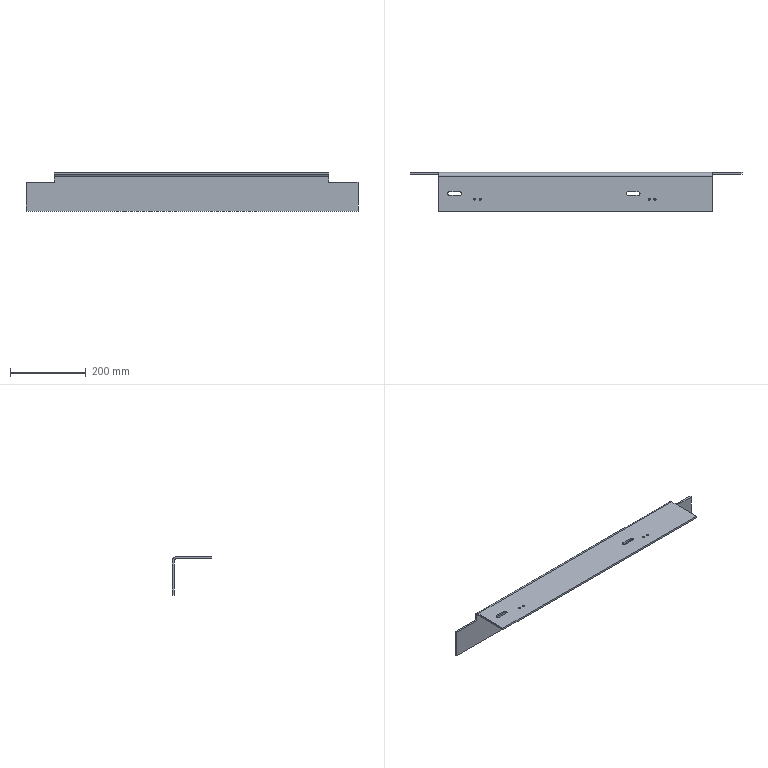Part | NX | 1 solid | 40 faces | box 874.4 x 103.1 x 101 mm | volume 761478 mm3 | plane 16 | cylinder 16 | cone 8 | commonest cylinder face diameters 5 x8 10 x7 20 x1
STEP:
#1=CARTESIAN_POINT('',(669.7,130.8,34.5));
#2=VERTEX_POINT('',#1);
#3=CARTESIAN_POINT('',(669.7,223.9,34.5));
#4=VERTEX_POINT('',#3);
#5=CARTESIAN_POINT('',(669.7,141.246,34.5));
#6=DIRECTION('',(0.,1.,0.));
#7=VECTOR('',#6,1000.);
#8=LINE('',#5,#7);
#9=EDGE_CURVE('',#2,#4,#8,.T.);
#10=ORIENTED_EDGE('',*,*,#9,.F.);
#11=CARTESIAN_POINT('',(669.7,130.8,29.5));
#12=VERTEX_POINT('',#11);
#13=CARTESIAN_POINT('',(669.7,130.8,29.5));
#14=DIRECTION('',(0.,0.,1.));
#15=VECTOR('',#14,1000.);
#16=LINE('',#13,#15);
#17=EDGE_CURVE('',#12,#2,#16,.T.);
#18=ORIENTED_EDGE('',*,*,#17,.F.);
#19=CARTESIAN_POINT('',(669.7,223.9,29.5));
#20=VERTEX_POINT('',#19);
#21=CARTESIAN_POINT('',(669.7,141.246,29.5));
#22=DIRECTION('',(0.,1.,0.));
#23=VECTOR('',#22,1000.);
#24=LINE('',#21,#23);
#25=EDGE_CURVE('',#12,#20,#24,.T.);
#26=ORIENTED_EDGE('',*,*,#25,.T.);
#27=CARTESIAN_POINT('',(669.7,228.9,24.5));
#28=VERTEX_POINT('',#27);
#29=CARTESIAN_POINT('',(669.7,223.9,24.5));
#30=DIRECTION('',(1.,0.,0.));
#31=DIRECTION('',(0.,-1.,0.));
#32=AXIS2_PLACEMENT_3D('',#29,#30,#31);
#33=CIRCLE('',#32,5.);
#34=EDGE_CURVE('',#28,#20,#33,.T.);
#35=ORIENTED_EDGE('',*,*,#34,.F.);
#36=CARTESIAN_POINT('',(669.7,228.9,9.5));
#37=VERTEX_POINT('',#36);
#38=CARTESIAN_POINT('',(669.7,228.9,29.5));
#39=DIRECTION('',(0.,0.,-1.));
#40=VECTOR('',#39,1000.);
#41=LINE('',#38,#40);
#42=EDGE_CURVE('',#28,#37,#41,.T.);
#43=ORIENTED_EDGE('',*,*,#42,.T.);
#44=CARTESIAN_POINT('',(669.7,233.9,9.5));
#45=VERTEX_POINT('',#44);
#46=CARTESIAN_POINT('',(669.7,141.246,9.5));
#47=DIRECTION('',(0.,1.,0.));
#48=VECTOR('',#47,1000.);
#49=LINE('',#46,#48);
#50=EDGE_CURVE('',#37,#45,#49,.T.);
#51=ORIENTED_EDGE('',*,*,#50,.T.);
#52=CARTESIAN_POINT('',(669.7,233.9,24.5));
#53=VERTEX_POINT('',#52);
#54=CARTESIAN_POINT('',(669.7,233.9,29.5));
#55=DIRECTION('',(0.,0.,-1.));
#56=VECTOR('',#55,1000.);
#57=LINE('',#54,#56);
#58=EDGE_CURVE('',#53,#45,#57,.T.);
#59=ORIENTED_EDGE('',*,*,#58,.F.);
#60=CARTESIAN_POINT('',(669.7,223.9,24.5));
#61=DIRECTION('',(1.,0.,0.));
#62=DIRECTION('',(0.,-1.,0.));
#63=AXIS2_PLACEMENT_3D('',#60,#61,#62);
#64=CIRCLE('',#63,10.);
#65=EDGE_CURVE('',#53,#4,#64,.T.);
#66=ORIENTED_EDGE('',*,*,#65,.T.);
#67=EDGE_LOOP('',(#10,#18,#26,#35,#43,#51,#59,#66));
#68=FACE_BOUND('',#67,.T.);
#69=CARTESIAN_POINT('',(669.7,165.9,29.5));
#70=DIRECTION('',(1.,0.,0.));
#71=DIRECTION('',(0.,1.,0.));
#72=AXIS2_PLACEMENT_3D('',#69,#70,#71);
#73=PLANE('',#72);
#74=ADVANCED_FACE('',(#68),#73,.T.);
#75=CARTESIAN_POINT('',(-52.7,130.8,29.5));
#76=VERTEX_POINT('',#75);
#77=CARTESIAN_POINT('',(357.184,130.8,29.5));
#78=DIRECTION('',(1.,0.,0.));
#79=VECTOR('',#78,1000.);
#80=LINE('',#77,#79);
#81=EDGE_CURVE('',#76,#12,#80,.T.);
#82=ORIENTED_EDGE('',*,*,#81,.T.);
#83=ORIENTED_EDGE('',*,*,#17,.T.);
#84=CARTESIAN_POINT('',(-52.7,130.8,34.5));
#85=VERTEX_POINT('',#84);
#86=CARTESIAN_POINT('',(357.184,130.8,34.5));
#87=DIRECTION('',(1.,0.,0.));
#88=VECTOR('',#87,1000.);
#89=LINE('',#86,#88);
#90=EDGE_CURVE('',#85,#2,#89,.T.);
#91=ORIENTED_EDGE('',*,*,#90,.F.);
#92=CARTESIAN_POINT('',(-52.7,130.8,29.5));
#93=DIRECTION('',(0.,0.,-1.));
#94=VECTOR('',#93,1000.);
#95=LINE('',#92,#94);
#96=EDGE_CURVE('',#85,#76,#95,.T.);
#97=ORIENTED_EDGE('',*,*,#96,.T.);
#98=EDGE_LOOP('',(#82,#83,#91,#97));
#99=FACE_BOUND('',#98,.T.);
#100=CARTESIAN_POINT('',(364.7,130.8,29.5));
#101=DIRECTION('',(0.,-1.,0.));
#102=DIRECTION('',(0.,0.,-1.));
#103=AXIS2_PLACEMENT_3D('',#100,#101,#102);
#104=PLANE('',#103);
#105=ADVANCED_FACE('',(#99),#104,.T.);
#106=CARTESIAN_POINT('',(746.7,233.9,9.5));
#107=VERTEX_POINT('',#106);
#108=CARTESIAN_POINT('',(746.7,233.9,-66.5));
#109=VERTEX_POINT('',#108);
#110=CARTESIAN_POINT('',(746.7,233.9,29.5));
#111=DIRECTION('',(0.,0.,-1.));
#112=VECTOR('',#111,1000.);
#113=LINE('',#110,#112);
#114=EDGE_CURVE('',#107,#109,#113,.T.);
#115=ORIENTED_EDGE('',*,*,#114,.F.);
#116=CARTESIAN_POINT('',(746.7,228.9,9.5));
#117=VERTEX_POINT('',#116);
#118=CARTESIAN_POINT('',(746.7,141.246,9.5));
#119=DIRECTION('',(0.,-1.,0.));
#120=VECTOR('',#119,1000.);
#121=LINE('',#118,#120);
#122=EDGE_CURVE('',#107,#117,#121,.T.);
#123=ORIENTED_EDGE('',*,*,#122,.T.);
#124=CARTESIAN_POINT('',(746.7,228.9,-66.5));
#125=VERTEX_POINT('',#124);
#126=CARTESIAN_POINT('',(746.7,228.9,29.5));
#127=DIRECTION('',(0.,0.,-1.));
#128=VECTOR('',#127,1000.);
#129=LINE('',#126,#128);
#130=EDGE_CURVE('',#117,#125,#129,.T.);
#131=ORIENTED_EDGE('',*,*,#130,.T.);
#132=CARTESIAN_POINT('',(746.7,141.246,-66.5));
#133=DIRECTION('',(0.,1.,0.));
#134=VECTOR('',#133,1000.);
#135=LINE('',#132,#134);
#136=EDGE_CURVE('',#125,#109,#135,.T.);
#137=ORIENTED_EDGE('',*,*,#136,.T.);
#138=EDGE_LOOP('',(#115,#123,#131,#137));
#139=FACE_BOUND('',#138,.T.);
#140=CARTESIAN_POINT('',(746.7,230.407,-49.685));
#141=DIRECTION('',(1.,0.,0.));
#142=DIRECTION('',(0.,1.,0.));
#143=AXIS2_PLACEMENT_3D('',#140,#141,#142);
#144=PLANE('',#143);
#145=ADVANCED_FACE('',(#139),#144,.T.);
#146=ORIENTED_EDGE('',*,*,#50,.F.);
#147=CARTESIAN_POINT('',(357.184,228.9,9.5));
#148=DIRECTION('',(1.,0.,0.));
#149=VECTOR('',#148,1000.);
#150=LINE('',#147,#149);
#151=EDGE_CURVE('',#37,#117,#150,.T.);
#152=ORIENTED_EDGE('',*,*,#151,.T.);
#153=ORIENTED_EDGE('',*,*,#122,.F.);
#154=CARTESIAN_POINT('',(357.184,233.9,9.5));
#155=DIRECTION('',(1.,0.,0.));
#156=VECTOR('',#155,1000.);
#157=LINE('',#154,#156);
#158=EDGE_CURVE('',#45,#107,#157,.T.);
#159=ORIENTED_EDGE('',*,*,#158,.F.);
#160=EDGE_LOOP('',(#146,#152,#153,#159));
#161=FACE_BOUND('',#160,.T.);
#162=CARTESIAN_POINT('',(671.7,228.9,9.5));
#163=DIRECTION('',(0.,0.,1.));
#164=DIRECTION('',(1.,0.,0.));
#165=AXIS2_PLACEMENT_3D('',#162,#163,#164);
#166=PLANE('',#165);
#167=ADVANCED_FACE('',(#161),#166,.T.);
#168=ORIENTED_EDGE('',*,*,#9,.T.);
#169=CARTESIAN_POINT('',(-52.7,223.9,34.5));
#170=VERTEX_POINT('',#169);
#171=CARTESIAN_POINT('',(357.184,223.9,34.5));
#172=DIRECTION('',(1.,0.,0.));
#173=VECTOR('',#172,1000.);
#174=LINE('',#171,#173);
#175=EDGE_CURVE('',#170,#4,#174,.T.);
#176=ORIENTED_EDGE('',*,*,#175,.F.);
#177=CARTESIAN_POINT('',(-52.7,233.9,34.5));
#178=DIRECTION('',(0.,1.,0.));
#179=VECTOR('',#178,1000.);
#180=LINE('',#177,#179);
#181=EDGE_CURVE('',#85,#170,#180,.T.);
#182=ORIENTED_EDGE('',*,*,#181,.F.);
#183=ORIENTED_EDGE('',*,*,#90,.T.);
#184=EDGE_LOOP('',(#168,#176,#182,#183));
#185=FACE_BOUND('',#184,.T.);
#186=CARTESIAN_POINT('',(39.8,163.7,34.5));
#187=VERTEX_POINT('',#186);
#188=CARTESIAN_POINT('',(45.2,163.7,34.5));
#189=VERTEX_POINT('',#188);
#190=CARTESIAN_POINT('',(42.5,163.7,34.5));
#191=DIRECTION('',(0.,0.,1.));
#192=DIRECTION('',(1.,0.,0.));
#193=AXIS2_PLACEMENT_3D('',#190,#191,#192);
#194=CIRCLE('',#193,2.7);
#195=EDGE_CURVE('',#187,#189,#194,.T.);
#196=ORIENTED_EDGE('',*,*,#195,.F.);
#197=CARTESIAN_POINT('',(42.5,163.7,34.5));
#198=DIRECTION('',(0.,0.,1.));
#199=DIRECTION('',(1.,0.,0.));
#200=AXIS2_PLACEMENT_3D('',#197,#198,#199);
#201=CIRCLE('',#200,2.7);
#202=EDGE_CURVE('',#189,#187,#201,.T.);
#203=ORIENTED_EDGE('',*,*,#202,.F.);
#204=EDGE_LOOP('',(#196,#203));
#205=FACE_BOUND('',#204,.T.);
#206=CARTESIAN_POINT('',(514.8,163.7,34.5));
#207=VERTEX_POINT('',#206);
#208=CARTESIAN_POINT('',(520.2,163.7,34.5));
#209=VERTEX_POINT('',#208);
#210=CARTESIAN_POINT('',(517.5,163.7,34.5));
#211=DIRECTION('',(0.,0.,1.));
#212=DIRECTION('',(1.,0.,0.));
#213=AXIS2_PLACEMENT_3D('',#210,#211,#212);
#214=CIRCLE('',#213,2.7);
#215=EDGE_CURVE('',#207,#209,#214,.T.);
#216=ORIENTED_EDGE('',*,*,#215,.F.);
#217=CARTESIAN_POINT('',(517.5,163.7,34.5));
#218=DIRECTION('',(0.,0.,1.));
#219=DIRECTION('',(1.,0.,0.));
#220=AXIS2_PLACEMENT_3D('',#217,#218,#219);
#221=CIRCLE('',#220,2.7);
#222=EDGE_CURVE('',#209,#207,#221,.T.);
#223=ORIENTED_EDGE('',*,*,#222,.F.);
#224=EDGE_LOOP('',(#216,#223));
#225=FACE_BOUND('',#224,.T.);
#226=CARTESIAN_POINT('',(54.8,163.7,34.5));
#227=VERTEX_POINT('',#226);
#228=CARTESIAN_POINT('',(60.2,163.7,34.5));
#229=VERTEX_POINT('',#228);
#230=CARTESIAN_POINT('',(57.5,163.7,34.5));
#231=DIRECTION('',(0.,0.,1.));
#232=DIRECTION('',(1.,0.,0.));
#233=AXIS2_PLACEMENT_3D('',#230,#231,#232);
#234=CIRCLE('',#233,2.7);
#235=EDGE_CURVE('',#227,#229,#234,.T.);
#236=ORIENTED_EDGE('',*,*,#235,.F.);
#237=CARTESIAN_POINT('',(57.5,163.7,34.5));
#238=DIRECTION('',(0.,0.,1.));
#239=DIRECTION('',(1.,0.,0.));
#240=AXIS2_PLACEMENT_3D('',#237,#238,#239);
#241=CIRCLE('',#240,2.7);
#242=EDGE_CURVE('',#229,#227,#241,.T.);
#243=ORIENTED_EDGE('',*,*,#242,.F.);
#244=EDGE_LOOP('',(#236,#243));
#245=FACE_BOUND('',#244,.T.);
#246=CARTESIAN_POINT('',(499.8,163.7,34.5));
#247=VERTEX_POINT('',#246);
#248=CARTESIAN_POINT('',(505.2,163.7,34.5));
#249=VERTEX_POINT('',#248);
#250=CARTESIAN_POINT('',(502.5,163.7,34.5));
#251=DIRECTION('',(0.,0.,1.));
#252=DIRECTION('',(1.,0.,0.));
#253=AXIS2_PLACEMENT_3D('',#250,#251,#252);
#254=CIRCLE('',#253,2.7);
#255=EDGE_CURVE('',#247,#249,#254,.T.);
#256=ORIENTED_EDGE('',*,*,#255,.F.);
#257=CARTESIAN_POINT('',(502.5,163.7,34.5));
#258=DIRECTION('',(0.,0.,1.));
#259=DIRECTION('',(1.,0.,0.));
#260=AXIS2_PLACEMENT_3D('',#257,#258,#259);
#261=CIRCLE('',#260,2.7);
#262=EDGE_CURVE('',#249,#247,#261,.T.);
#263=ORIENTED_EDGE('',*,*,#262,.F.);
#264=EDGE_LOOP('',(#256,#263));
#265=FACE_BOUND('',#264,.T.);
#266=CARTESIAN_POINT('',(3.125,173.2,34.5));
#267=VERTEX_POINT('',#266);
#268=CARTESIAN_POINT('',(8.125,178.2,34.5));
#269=VERTEX_POINT('',#268);
#270=CARTESIAN_POINT('',(3.125,178.2,34.5));
#271=DIRECTION('',(0.,0.,1.));
#272=DIRECTION('',(1.,0.,0.));
#273=AXIS2_PLACEMENT_3D('',#270,#271,#272);
#274=CIRCLE('',#273,5.);
#275=EDGE_CURVE('',#267,#269,#274,.T.);
#276=ORIENTED_EDGE('',*,*,#275,.F.);
#277=CARTESIAN_POINT('',(-23.125,173.2,34.5));
#278=VERTEX_POINT('',#277);
#279=CARTESIAN_POINT('',(357.184,173.2,34.5));
#280=DIRECTION('',(1.,0.,0.));
#281=VECTOR('',#280,1000.);
#282=LINE('',#279,#281);
#283=EDGE_CURVE('',#278,#267,#282,.T.);
#284=ORIENTED_EDGE('',*,*,#283,.F.);
#285=CARTESIAN_POINT('',(-23.125,183.2,34.5));
#286=VERTEX_POINT('',#285);
#287=CARTESIAN_POINT('',(-23.125,178.2,34.5));
#288=DIRECTION('',(0.,0.,1.));
#289=DIRECTION('',(1.,0.,0.));
#290=AXIS2_PLACEMENT_3D('',#287,#288,#289);
#291=CIRCLE('',#290,5.);
#292=EDGE_CURVE('',#286,#278,#291,.T.);
#293=ORIENTED_EDGE('',*,*,#292,.F.);
#294=CARTESIAN_POINT('',(3.125,183.2,34.5));
#295=VERTEX_POINT('',#294);
#296=CARTESIAN_POINT('',(357.184,183.2,34.5));
#297=DIRECTION('',(-1.,0.,0.));
#298=VECTOR('',#297,1000.);
#299=LINE('',#296,#298);
#300=EDGE_CURVE('',#295,#286,#299,.T.);
#301=ORIENTED_EDGE('',*,*,#300,.F.);
#302=CARTESIAN_POINT('',(3.125,178.2,34.5));
#303=DIRECTION('',(0.,0.,1.));
#304=DIRECTION('',(1.,0.,0.));
#305=AXIS2_PLACEMENT_3D('',#302,#303,#304);
#306=CIRCLE('',#305,5.);
#307=EDGE_CURVE('',#269,#295,#306,.T.);
#308=ORIENTED_EDGE('',*,*,#307,.F.);
#309=EDGE_LOOP('',(#276,#284,#293,#301,#308));
#310=FACE_BOUND('',#309,.T.);
#311=CARTESIAN_POINT('',(446.875,173.2,34.5));
#312=VERTEX_POINT('',#311);
#313=CARTESIAN_POINT('',(473.125,173.2,34.5));
#314=VERTEX_POINT('',#313);
#315=CARTESIAN_POINT('',(357.184,173.2,34.5));
#316=DIRECTION('',(1.,0.,0.));
#317=VECTOR('',#316,1000.);
#318=LINE('',#315,#317);
#319=EDGE_CURVE('',#312,#314,#318,.T.);
#320=ORIENTED_EDGE('',*,*,#319,.F.);
#321=CARTESIAN_POINT('',(446.875,183.2,34.5));
#322=VERTEX_POINT('',#321);
#323=CARTESIAN_POINT('',(446.875,178.2,34.5));
#324=DIRECTION('',(0.,0.,1.));
#325=DIRECTION('',(1.,0.,0.));
#326=AXIS2_PLACEMENT_3D('',#323,#324,#325);
#327=CIRCLE('',#326,5.);
#328=EDGE_CURVE('',#322,#312,#327,.T.);
#329=ORIENTED_EDGE('',*,*,#328,.F.);
#330=CARTESIAN_POINT('',(473.125,183.2,34.5));
#331=VERTEX_POINT('',#330);
#332=CARTESIAN_POINT('',(357.184,183.2,34.5));
#333=DIRECTION('',(-1.,0.,0.));
#334=VECTOR('',#333,1000.);
#335=LINE('',#332,#334);
#336=EDGE_CURVE('',#331,#322,#335,.T.);
#337=ORIENTED_EDGE('',*,*,#336,.F.);
#338=CARTESIAN_POINT('',(478.125,178.2,34.5));
#339=VERTEX_POINT('',#338);
#340=CARTESIAN_POINT('',(473.125,178.2,34.5));
#341=DIRECTION('',(0.,0.,1.));
#342=DIRECTION('',(1.,0.,0.));
#343=AXIS2_PLACEMENT_3D('',#340,#341,#342);
#344=CIRCLE('',#343,5.);
#345=EDGE_CURVE('',#339,#331,#344,.T.);
#346=ORIENTED_EDGE('',*,*,#345,.F.);
#347=CARTESIAN_POINT('',(473.125,178.2,34.5));
#348=DIRECTION('',(0.,0.,1.));
#349=DIRECTION('',(1.,0.,0.));
#350=AXIS2_PLACEMENT_3D('',#347,#348,#349);
#351=CIRCLE('',#350,5.);
#352=EDGE_CURVE('',#314,#339,#351,.T.);
#353=ORIENTED_EDGE('',*,*,#352,.F.);
#354=EDGE_LOOP('',(#320,#329,#337,#346,#353));
#355=FACE_BOUND('',#354,.T.);
#356=CARTESIAN_POINT('',(-52.7,233.9,34.5));
#357=DIRECTION('',(0.,0.,1.));
#358=DIRECTION('',(1.,0.,0.));
#359=AXIS2_PLACEMENT_3D('',#356,#357,#358);
#360=PLANE('',#359);
#361=ADVANCED_FACE('',(#185,#205,#225,#245,#265,#310,#355),#360,.T.);
#362=CARTESIAN_POINT('',(478.125,178.2,29.5));
#363=VERTEX_POINT('',#362);
#364=CARTESIAN_POINT('',(478.125,178.2,-76.6));
#365=DIRECTION('',(0.,0.,1.));
#366=VECTOR('',#365,1000.);
#367=LINE('',#364,#366);
#368=EDGE_CURVE('',#363,#339,#367,.T.);
#369=ORIENTED_EDGE('',*,*,#368,.F.);
#370=CARTESIAN_POINT('',(473.125,173.2,29.5));
#371=VERTEX_POINT('',#370);
#372=CARTESIAN_POINT('',(473.125,178.2,29.5));
#373=DIRECTION('',(0.,0.,1.));
#374=DIRECTION('',(1.,0.,0.));
#375=AXIS2_PLACEMENT_3D('',#372,#373,#374);
#376=CIRCLE('',#375,5.);
#377=EDGE_CURVE('',#371,#363,#376,.T.);
#378=ORIENTED_EDGE('',*,*,#377,.F.);
#379=CARTESIAN_POINT('',(473.125,173.2,-76.6));
#380=DIRECTION('',(0.,0.,1.));
#381=VECTOR('',#380,1000.);
#382=LINE('',#379,#381);
#383=EDGE_CURVE('',#371,#314,#382,.T.);
#384=ORIENTED_EDGE('',*,*,#383,.T.);
#385=ORIENTED_EDGE('',*,*,#352,.T.);
#386=EDGE_LOOP('',(#369,#378,#384,#385));
#387=FACE_BOUND('',#386,.T.);
#388=CARTESIAN_POINT('',(473.125,178.2,-76.6));
#389=DIRECTION('',(0.,0.,1.));
#390=DIRECTION('',(1.,0.,0.));
#391=AXIS2_PLACEMENT_3D('',#388,#389,#390);
#392=CYLINDRICAL_SURFACE('',#391,5.);
#393=ADVANCED_FACE('',(#387),#392,.F.);
#394=CARTESIAN_POINT('',(-127.7,233.9,-66.5));
#395=VERTEX_POINT('',#394);
#396=CARTESIAN_POINT('',(357.184,233.9,-66.5));
#397=DIRECTION('',(-1.,0.,0.));
#398=VECTOR('',#397,1000.);
#399=LINE('',#396,#398);
#400=EDGE_CURVE('',#109,#395,#399,.T.);
#401=ORIENTED_EDGE('',*,*,#400,.F.);
#402=ORIENTED_EDGE('',*,*,#136,.F.);
#403=CARTESIAN_POINT('',(-127.7,228.9,-66.5));
#404=VERTEX_POINT('',#403);
#405=CARTESIAN_POINT('',(357.184,228.9,-66.5));
#406=DIRECTION('',(-1.,0.,0.));
#407=VECTOR('',#406,1000.);
#408=LINE('',#405,#407);
#409=EDGE_CURVE('',#125,#404,#408,.T.);
#410=ORIENTED_EDGE('',*,*,#409,.T.);
#411=CARTESIAN_POINT('',(-127.7,141.246,-66.5));
#412=DIRECTION('',(0.,-1.,0.));
#413=VECTOR('',#412,1000.);
#414=LINE('',#411,#413);
#415=EDGE_CURVE('',#395,#404,#414,.T.);
#416=ORIENTED_EDGE('',*,*,#415,.F.);
#417=EDGE_LOOP('',(#401,#402,#410,#416));
#418=FACE_BOUND('',#417,.T.);
#419=CARTESIAN_POINT('',(671.7,233.9,-66.5));
#420=DIRECTION('',(0.,0.,-1.));
#421=DIRECTION('',(0.,-1.,0.));
#422=AXIS2_PLACEMENT_3D('',#419,#420,#421);
#423=PLANE('',#422);
#424=ADVANCED_FACE('',(#418),#423,.T.);
#425=CARTESIAN_POINT('',(-52.7,233.9,24.5));
#426=VERTEX_POINT('',#425);
#427=CARTESIAN_POINT('',(357.184,233.9,24.5));
#428=DIRECTION('',(1.,0.,0.));
#429=VECTOR('',#428,1000.);
#430=LINE('',#427,#429);
#431=EDGE_CURVE('',#426,#53,#430,.T.);
#432=ORIENTED_EDGE('',*,*,#431,.T.);
#433=ORIENTED_EDGE('',*,*,#58,.T.);
#434=ORIENTED_EDGE('',*,*,#158,.T.);
#435=ORIENTED_EDGE('',*,*,#114,.T.);
#436=ORIENTED_EDGE('',*,*,#400,.T.);
#437=CARTESIAN_POINT('',(-127.7,233.9,9.5));
#438=VERTEX_POINT('',#437);
#439=CARTESIAN_POINT('',(-127.7,233.9,29.5));
#440=DIRECTION('',(0.,0.,-1.));
#441=VECTOR('',#440,1000.);
#442=LINE('',#439,#441);
#443=EDGE_CURVE('',#438,#395,#442,.T.);
#444=ORIENTED_EDGE('',*,*,#443,.F.);
#445=CARTESIAN_POINT('',(-52.7,233.9,9.5));
#446=VERTEX_POINT('',#445);
#447=CARTESIAN_POINT('',(-52.7,233.9,9.5));
#448=DIRECTION('',(-1.,0.,0.));
#449=VECTOR('',#448,1000.);
#450=LINE('',#447,#449);
#451=EDGE_CURVE('',#446,#438,#450,.T.);
#452=ORIENTED_EDGE('',*,*,#451,.F.);
#453=CARTESIAN_POINT('',(-52.7,233.9,29.5));
#454=DIRECTION('',(0.,0.,-1.));
#455=VECTOR('',#454,1000.);
#456=LINE('',#453,#455);
#457=EDGE_CURVE('',#426,#446,#456,.T.);
#458=ORIENTED_EDGE('',*,*,#457,.F.);
#459=EDGE_LOOP('',(#432,#433,#434,#435,#436,#444,#452,#458));
#460=FACE_BOUND('',#459,.T.);
#461=CARTESIAN_POINT('',(-52.7,233.9,24.907));
#462=DIRECTION('',(0.,1.,0.));
#463=DIRECTION('',(1.,0.,0.));
#464=AXIS2_PLACEMENT_3D('',#461,#462,#463);
#465=PLANE('',#464);
#466=ADVANCED_FACE('',(#460),#465,.T.);
#467=ORIENTED_EDGE('',*,*,#175,.T.);
#468=ORIENTED_EDGE('',*,*,#65,.F.);
#469=ORIENTED_EDGE('',*,*,#431,.F.);
#470=CARTESIAN_POINT('',(-52.7,223.9,24.5));
#471=DIRECTION('',(-1.,0.,0.));
#472=DIRECTION('',(0.,0.,1.));
#473=AXIS2_PLACEMENT_3D('',#470,#471,#472);
#474=CIRCLE('',#473,10.);
#475=EDGE_CURVE('',#170,#426,#474,.T.);
#476=ORIENTED_EDGE('',*,*,#475,.F.);
#477=EDGE_LOOP('',(#467,#468,#469,#476));
#478=FACE_BOUND('',#477,.T.);
#479=CARTESIAN_POINT('',(671.7,223.9,24.5));
#480=DIRECTION('',(1.,0.,0.));
#481=DIRECTION('',(0.,-1.,0.));
#482=AXIS2_PLACEMENT_3D('',#479,#480,#481);
#483=CYLINDRICAL_SURFACE('',#482,10.);
#484=ADVANCED_FACE('',(#478),#483,.T.);
#485=CARTESIAN_POINT('',(-52.7,228.9,9.5));
#486=VERTEX_POINT('',#485);
#487=CARTESIAN_POINT('',(-52.7,141.246,9.5));
#488=DIRECTION('',(0.,1.,0.));
#489=VECTOR('',#488,1000.);
#490=LINE('',#487,#489);
#491=EDGE_CURVE('',#486,#446,#490,.T.);
#492=ORIENTED_EDGE('',*,*,#491,.F.);
#493=CARTESIAN_POINT('',(-52.7,228.9,24.5));
#494=VERTEX_POINT('',#493);
#495=CARTESIAN_POINT('',(-52.7,228.9,29.5));
#496=DIRECTION('',(0.,0.,1.));
#497=VECTOR('',#496,1000.);
#498=LINE('',#495,#497);
#499=EDGE_CURVE('',#486,#494,#498,.T.);
#500=ORIENTED_EDGE('',*,*,#499,.T.);
#501=CARTESIAN_POINT('',(-52.7,223.9,29.5));
#502=VERTEX_POINT('',#501);
#503=CARTESIAN_POINT('',(-52.7,223.9,24.5));
#504=DIRECTION('',(1.,0.,0.));
#505=DIRECTION('',(0.,1.,0.));
#506=AXIS2_PLACEMENT_3D('',#503,#504,#505);
#507=CIRCLE('',#506,5.);
#508=EDGE_CURVE('',#494,#502,#507,.T.);
#509=ORIENTED_EDGE('',*,*,#508,.T.);
#510=CARTESIAN_POINT('',(-52.7,141.246,29.5));
#511=DIRECTION('',(0.,-1.,0.));
#512=VECTOR('',#511,1000.);
#513=LINE('',#510,#512);
#514=EDGE_CURVE('',#502,#76,#513,.T.);
#515=ORIENTED_EDGE('',*,*,#514,.T.);
#516=ORIENTED_EDGE('',*,*,#96,.F.);
#517=ORIENTED_EDGE('',*,*,#181,.T.);
#518=ORIENTED_EDGE('',*,*,#475,.T.);
#519=ORIENTED_EDGE('',*,*,#457,.T.);
#520=EDGE_LOOP('',(#492,#500,#509,#515,#516,#517,#518,#519));
#521=FACE_BOUND('',#520,.T.);
#522=CARTESIAN_POINT('',(-52.7,233.9,-60.5));
#523=DIRECTION('',(-1.,0.,0.));
#524=DIRECTION('',(0.,0.,1.));
#525=AXIS2_PLACEMENT_3D('',#522,#523,#524);
#526=PLANE('',#525);
#527=ADVANCED_FACE('',(#521),#526,.T.);
#528=ORIENTED_EDGE('',*,*,#319,.T.);
#529=ORIENTED_EDGE('',*,*,#383,.F.);
#530=CARTESIAN_POINT('',(446.875,173.2,29.5));
#531=VERTEX_POINT('',#530);
#532=CARTESIAN_POINT('',(357.184,173.2,29.5));
#533=DIRECTION('',(1.,0.,0.));
#534=VECTOR('',#533,1000.);
#535=LINE('',#532,#534);
#536=EDGE_CURVE('',#531,#371,#535,.T.);
#537=ORIENTED_EDGE('',*,*,#536,.F.);
#538=CARTESIAN_POINT('',(446.875,173.2,-76.6));
#539=DIRECTION('',(0.,0.,1.));
#540=VECTOR('',#539,1000.);
#541=LINE('',#538,#540);
#542=EDGE_CURVE('',#531,#312,#541,.T.);
#543=ORIENTED_EDGE('',*,*,#542,.T.);
#544=EDGE_LOOP('',(#528,#529,#537,#543));
#545=FACE_BOUND('',#544,.T.);
#546=CARTESIAN_POINT('',(473.125,173.2,-76.6));
#547=DIRECTION('',(0.,-1.,0.));
#548=DIRECTION('',(0.,0.,-1.));
#549=AXIS2_PLACEMENT_3D('',#546,#547,#548);
#550=PLANE('',#549);
#551=ADVANCED_FACE('',(#545),#550,.F.);
#552=ORIENTED_EDGE('',*,*,#491,.T.);
#553=ORIENTED_EDGE('',*,*,#451,.T.);
#554=CARTESIAN_POINT('',(-127.7,228.9,9.5));
#555=VERTEX_POINT('',#554);
#556=CARTESIAN_POINT('',(-127.7,141.246,9.5));
#557=DIRECTION('',(0.,-1.,0.));
#558=VECTOR('',#557,1000.);
#559=LINE('',#556,#558);
#560=EDGE_CURVE('',#438,#555,#559,.T.);
#561=ORIENTED_EDGE('',*,*,#560,.T.);
#562=CARTESIAN_POINT('',(-52.7,228.9,9.5));
#563=DIRECTION('',(-1.,0.,0.));
#564=VECTOR('',#563,1000.);
#565=LINE('',#562,#564);
#566=EDGE_CURVE('',#486,#555,#565,.T.);
#567=ORIENTED_EDGE('',*,*,#566,.F.);
#568=EDGE_LOOP('',(#552,#553,#561,#567));
#569=FACE_BOUND('',#568,.T.);
#570=CARTESIAN_POINT('',(-52.7,233.9,9.5));
#571=DIRECTION('',(0.,0.,1.));
#572=DIRECTION('',(1.,0.,0.));
#573=AXIS2_PLACEMENT_3D('',#570,#571,#572);
#574=PLANE('',#573);
#575=ADVANCED_FACE('',(#569),#574,.T.);
#576=ORIENTED_EDGE('',*,*,#415,.T.);
#577=CARTESIAN_POINT('',(-127.7,228.9,29.5));
#578=DIRECTION('',(0.,0.,-1.));
#579=VECTOR('',#578,1000.);
#580=LINE('',#577,#579);
#581=EDGE_CURVE('',#555,#404,#580,.T.);
#582=ORIENTED_EDGE('',*,*,#581,.F.);
#583=ORIENTED_EDGE('',*,*,#560,.F.);
#584=ORIENTED_EDGE('',*,*,#443,.T.);
#585=EDGE_LOOP('',(#576,#582,#583,#584));
#586=FACE_BOUND('',#585,.T.);
#587=CARTESIAN_POINT('',(-127.7,231.365,-31.462));
#588=DIRECTION('',(-1.,0.,0.));
#589=DIRECTION('',(0.,0.,1.));
#590=AXIS2_PLACEMENT_3D('',#587,#588,#589);
#591=PLANE('',#590);
#592=ADVANCED_FACE('',(#586),#591,.T.);
#593=CARTESIAN_POINT('',(500.,163.7,34.3));
#594=VERTEX_POINT('',#593);
#595=CARTESIAN_POINT('',(505.,163.7,34.3));
#596=VERTEX_POINT('',#595);
#597=CARTESIAN_POINT('',(502.5,163.7,34.3));
#598=DIRECTION('',(0.,0.,1.));
#599=DIRECTION('',(1.,0.,0.));
#600=AXIS2_PLACEMENT_3D('',#597,#598,#599);
#601=CIRCLE('',#600,2.5);
#602=EDGE_CURVE('',#594,#596,#601,.T.);
#603=ORIENTED_EDGE('',*,*,#602,.T.);
#604=CARTESIAN_POINT('',(505.,163.7,29.5));
#605=VERTEX_POINT('',#604);
#606=CARTESIAN_POINT('',(505.,163.7,34.5));
#607=DIRECTION('',(0.,0.,1.));
#608=VECTOR('',#607,1000.);
#609=LINE('',#606,#608);
#610=EDGE_CURVE('',#605,#596,#609,.T.);
#611=ORIENTED_EDGE('',*,*,#610,.F.);
#612=CARTESIAN_POINT('',(500.,163.7,29.5));
#613=VERTEX_POINT('',#612);
#614=CARTESIAN_POINT('',(502.5,163.7,29.5));
#615=DIRECTION('',(0.,0.,1.));
#616=DIRECTION('',(1.,0.,0.));
#617=AXIS2_PLACEMENT_3D('',#614,#615,#616);
#618=CIRCLE('',#617,2.5);
#619=EDGE_CURVE('',#613,#605,#618,.T.);
#620=ORIENTED_EDGE('',*,*,#619,.F.);
#621=CARTESIAN_POINT('',(500.,163.7,34.5));
#622=DIRECTION('',(0.,0.,1.));
#623=VECTOR('',#622,1000.);
#624=LINE('',#621,#623);
#625=EDGE_CURVE('',#613,#594,#624,.T.);
#626=ORIENTED_EDGE('',*,*,#625,.T.);
#627=EDGE_LOOP('',(#603,#611,#620,#626));
#628=FACE_BOUND('',#627,.T.);
#629=CARTESIAN_POINT('',(502.5,163.7,34.5));
#630=DIRECTION('',(0.,0.,1.));
#631=DIRECTION('',(1.,0.,0.));
#632=AXIS2_PLACEMENT_3D('',#629,#630,#631);
#633=CYLINDRICAL_SURFACE('',#632,2.5);
#634=ADVANCED_FACE('',(#628),#633,.F.);
#635=ORIENTED_EDGE('',*,*,#602,.F.);
#636=CARTESIAN_POINT('',(500.,163.7,34.3));
#637=DIRECTION('',(-0.7071,0.,0.7071));
#638=VECTOR('',#637,1000.);
#639=LINE('',#636,#638);
#640=EDGE_CURVE('',#594,#247,#639,.T.);
#641=ORIENTED_EDGE('',*,*,#640,.T.);
#642=ORIENTED_EDGE('',*,*,#255,.T.);
#643=CARTESIAN_POINT('',(505.,163.7,34.3));
#644=DIRECTION('',(0.7071,0.,0.7071));
#645=VECTOR('',#644,1000.);
#646=LINE('',#643,#645);
#647=EDGE_CURVE('',#596,#249,#646,.T.);
#648=ORIENTED_EDGE('',*,*,#647,.F.);
#649=EDGE_LOOP('',(#635,#641,#642,#648));
#650=FACE_BOUND('',#649,.T.);
#651=CARTESIAN_POINT('',(502.5,163.7,34.3));
#652=DIRECTION('',(0.,0.,1.));
#653=DIRECTION('',(1.,0.,0.));
#654=AXIS2_PLACEMENT_3D('',#651,#652,#653);
#655=CONICAL_SURFACE('',#654,2.5,0.7854);
#656=ADVANCED_FACE('',(#650),#655,.F.);
#657=CARTESIAN_POINT('',(40.,163.7,34.3));
#658=VERTEX_POINT('',#657);
#659=CARTESIAN_POINT('',(45.,163.7,34.3));
#660=VERTEX_POINT('',#659);
#661=CARTESIAN_POINT('',(42.5,163.7,34.3));
#662=DIRECTION('',(0.,0.,1.));
#663=DIRECTION('',(1.,0.,0.));
#664=AXIS2_PLACEMENT_3D('',#661,#662,#663);
#665=CIRCLE('',#664,2.5);
#666=EDGE_CURVE('',#658,#660,#665,.T.);
#667=ORIENTED_EDGE('',*,*,#666,.T.);
#668=CARTESIAN_POINT('',(45.,163.7,29.5));
#669=VERTEX_POINT('',#668);
#670=CARTESIAN_POINT('',(45.,163.7,34.5));
#671=DIRECTION('',(0.,0.,1.));
#672=VECTOR('',#671,1000.);
#673=LINE('',#670,#672);
#674=EDGE_CURVE('',#669,#660,#673,.T.);
#675=ORIENTED_EDGE('',*,*,#674,.F.);
#676=CARTESIAN_POINT('',(40.,163.7,29.5));
#677=VERTEX_POINT('',#676);
#678=CARTESIAN_POINT('',(42.5,163.7,29.5));
#679=DIRECTION('',(0.,0.,1.));
#680=DIRECTION('',(1.,0.,0.));
#681=AXIS2_PLACEMENT_3D('',#678,#679,#680);
#682=CIRCLE('',#681,2.5);
#683=EDGE_CURVE('',#677,#669,#682,.T.);
#684=ORIENTED_EDGE('',*,*,#683,.F.);
#685=CARTESIAN_POINT('',(40.,163.7,34.5));
#686=DIRECTION('',(0.,0.,1.));
#687=VECTOR('',#686,1000.);
#688=LINE('',#685,#687);
#689=EDGE_CURVE('',#677,#658,#688,.T.);
#690=ORIENTED_EDGE('',*,*,#689,.T.);
#691=EDGE_LOOP('',(#667,#675,#684,#690));
#692=FACE_BOUND('',#691,.T.);
#693=CARTESIAN_POINT('',(42.5,163.7,34.5));
#694=DIRECTION('',(0.,0.,1.));
#695=DIRECTION('',(1.,0.,0.));
#696=AXIS2_PLACEMENT_3D('',#693,#694,#695);
#697=CYLINDRICAL_SURFACE('',#696,2.5);
#698=ADVANCED_FACE('',(#692),#697,.F.);
#699=ORIENTED_EDGE('',*,*,#666,.F.);
#700=CARTESIAN_POINT('',(40.,163.7,34.3));
#701=DIRECTION('',(-0.7071,0.,0.7071));
#702=VECTOR('',#701,1000.);
#703=LINE('',#700,#702);
#704=EDGE_CURVE('',#658,#187,#703,.T.);
#705=ORIENTED_EDGE('',*,*,#704,.T.);
#706=ORIENTED_EDGE('',*,*,#195,.T.);
#707=CARTESIAN_POINT('',(45.,163.7,34.3));
#708=DIRECTION('',(0.7071,0.,0.7071));
#709=VECTOR('',#708,1000.);
#710=LINE('',#707,#709);
#711=EDGE_CURVE('',#660,#189,#710,.T.);
#712=ORIENTED_EDGE('',*,*,#711,.F.);
#713=EDGE_LOOP('',(#699,#705,#706,#712));
#714=FACE_BOUND('',#713,.T.);
#715=CARTESIAN_POINT('',(42.5,163.7,34.3));
#716=DIRECTION('',(0.,0.,1.));
#717=DIRECTION('',(1.,0.,0.));
#718=AXIS2_PLACEMENT_3D('',#715,#716,#717);
#719=CONICAL_SURFACE('',#718,2.5,0.7854);
#720=ADVANCED_FACE('',(#714),#719,.F.);
#721=CARTESIAN_POINT('',(55.,163.7,34.3));
#722=VERTEX_POINT('',#721);
#723=CARTESIAN_POINT('',(60.,163.7,34.3));
#724=VERTEX_POINT('',#723);
#725=CARTESIAN_POINT('',(57.5,163.7,34.3));
#726=DIRECTION('',(0.,0.,1.));
#727=DIRECTION('',(1.,0.,0.));
#728=AXIS2_PLACEMENT_3D('',#725,#726,#727);
#729=CIRCLE('',#728,2.5);
#730=EDGE_CURVE('',#722,#724,#729,.T.);
#731=ORIENTED_EDGE('',*,*,#730,.T.);
#732=CARTESIAN_POINT('',(60.,163.7,29.5));
#733=VERTEX_POINT('',#732);
#734=CARTESIAN_POINT('',(60.,163.7,34.5));
#735=DIRECTION('',(0.,0.,1.));
#736=VECTOR('',#735,1000.);
#737=LINE('',#734,#736);
#738=EDGE_CURVE('',#733,#724,#737,.T.);
#739=ORIENTED_EDGE('',*,*,#738,.F.);
#740=CARTESIAN_POINT('',(55.,163.7,29.5));
#741=VERTEX_POINT('',#740);
#742=CARTESIAN_POINT('',(57.5,163.7,29.5));
#743=DIRECTION('',(0.,0.,1.));
#744=DIRECTION('',(1.,0.,0.));
#745=AXIS2_PLACEMENT_3D('',#742,#743,#744);
#746=CIRCLE('',#745,2.5);
#747=EDGE_CURVE('',#741,#733,#746,.T.);
#748=ORIENTED_EDGE('',*,*,#747,.F.);
#749=CARTESIAN_POINT('',(55.,163.7,34.5));
#750=DIRECTION('',(0.,0.,1.));
#751=VECTOR('',#750,1000.);
#752=LINE('',#749,#751);
#753=EDGE_CURVE('',#741,#722,#752,.T.);
#754=ORIENTED_EDGE('',*,*,#753,.T.);
#755=EDGE_LOOP('',(#731,#739,#748,#754));
#756=FACE_BOUND('',#755,.T.);
#757=CARTESIAN_POINT('',(57.5,163.7,34.5));
#758=DIRECTION('',(0.,0.,1.));
#759=DIRECTION('',(1.,0.,0.));
#760=AXIS2_PLACEMENT_3D('',#757,#758,#759);
#761=CYLINDRICAL_SURFACE('',#760,2.5);
#762=ADVANCED_FACE('',(#756),#761,.F.);
#763=ORIENTED_EDGE('',*,*,#730,.F.);
#764=CARTESIAN_POINT('',(55.,163.7,34.3));
#765=DIRECTION('',(-0.7071,0.,0.7071));
#766=VECTOR('',#765,1000.);
#767=LINE('',#764,#766);
#768=EDGE_CURVE('',#722,#227,#767,.T.);
#769=ORIENTED_EDGE('',*,*,#768,.T.);
#770=ORIENTED_EDGE('',*,*,#235,.T.);
#771=CARTESIAN_POINT('',(60.,163.7,34.3));
#772=DIRECTION('',(0.7071,0.,0.7071));
#773=VECTOR('',#772,1000.);
#774=LINE('',#771,#773);
#775=EDGE_CURVE('',#724,#229,#774,.T.);
#776=ORIENTED_EDGE('',*,*,#775,.F.);
#777=EDGE_LOOP('',(#763,#769,#770,#776));
#778=FACE_BOUND('',#777,.T.);
#779=CARTESIAN_POINT('',(57.5,163.7,34.3));
#780=DIRECTION('',(0.,0.,1.));
#781=DIRECTION('',(1.,0.,0.));
#782=AXIS2_PLACEMENT_3D('',#779,#780,#781);
#783=CONICAL_SURFACE('',#782,2.5,0.7854);
#784=ADVANCED_FACE('',(#778),#783,.F.);
#785=CARTESIAN_POINT('',(3.125,183.2,29.5));
#786=VERTEX_POINT('',#785);
#787=CARTESIAN_POINT('',(-23.125,183.2,29.5));
#788=VERTEX_POINT('',#787);
#789=CARTESIAN_POINT('',(357.184,183.2,29.5));
#790=DIRECTION('',(-1.,0.,0.));
#791=VECTOR('',#790,1000.);
#792=LINE('',#789,#791);
#793=EDGE_CURVE('',#786,#788,#792,.T.);
#794=ORIENTED_EDGE('',*,*,#793,.F.);
#795=CARTESIAN_POINT('',(3.125,183.2,-76.6));
#796=DIRECTION('',(0.,0.,1.));
#797=VECTOR('',#796,1000.);
#798=LINE('',#795,#797);
#799=EDGE_CURVE('',#786,#295,#798,.T.);
#800=ORIENTED_EDGE('',*,*,#799,.T.);
#801=ORIENTED_EDGE('',*,*,#300,.T.);
#802=CARTESIAN_POINT('',(-23.125,183.2,-76.6));
#803=DIRECTION('',(0.,0.,1.));
#804=VECTOR('',#803,1000.);
#805=LINE('',#802,#804);
#806=EDGE_CURVE('',#788,#286,#805,.T.);
#807=ORIENTED_EDGE('',*,*,#806,.F.);
#808=EDGE_LOOP('',(#794,#800,#801,#807));
#809=FACE_BOUND('',#808,.T.);
#810=CARTESIAN_POINT('',(-23.125,183.2,-76.6));
#811=DIRECTION('',(0.,1.,0.));
#812=DIRECTION('',(1.,0.,0.));
#813=AXIS2_PLACEMENT_3D('',#810,#811,#812);
#814=PLANE('',#813);
#815=ADVANCED_FACE('',(#809),#814,.F.);
#816=CARTESIAN_POINT('',(-23.125,173.2,29.5));
#817=VERTEX_POINT('',#816);
#818=CARTESIAN_POINT('',(-23.125,178.2,29.5));
#819=DIRECTION('',(0.,0.,1.));
#820=DIRECTION('',(1.,0.,0.));
#821=AXIS2_PLACEMENT_3D('',#818,#819,#820);
#822=CIRCLE('',#821,5.);
#823=EDGE_CURVE('',#788,#817,#822,.T.);
#824=ORIENTED_EDGE('',*,*,#823,.F.);
#825=ORIENTED_EDGE('',*,*,#806,.T.);
#826=ORIENTED_EDGE('',*,*,#292,.T.);
#827=CARTESIAN_POINT('',(-23.125,173.2,-76.6));
#828=DIRECTION('',(0.,0.,1.));
#829=VECTOR('',#828,1000.);
#830=LINE('',#827,#829);
#831=EDGE_CURVE('',#817,#278,#830,.T.);
#832=ORIENTED_EDGE('',*,*,#831,.F.);
#833=EDGE_LOOP('',(#824,#825,#826,#832));
#834=FACE_BOUND('',#833,.T.);
#835=CARTESIAN_POINT('',(-23.125,178.2,-76.6));
#836=DIRECTION('',(0.,0.,1.));
#837=DIRECTION('',(1.,0.,0.));
#838=AXIS2_PLACEMENT_3D('',#835,#836,#837);
#839=CYLINDRICAL_SURFACE('',#838,5.);
#840=ADVANCED_FACE('',(#834),#839,.F.);
#841=CARTESIAN_POINT('',(3.125,173.2,29.5));
#842=VERTEX_POINT('',#841);
#843=CARTESIAN_POINT('',(357.184,173.2,29.5));
#844=DIRECTION('',(1.,0.,0.));
#845=VECTOR('',#844,1000.);
#846=LINE('',#843,#845);
#847=EDGE_CURVE('',#817,#842,#846,.T.);
#848=ORIENTED_EDGE('',*,*,#847,.F.);
#849=ORIENTED_EDGE('',*,*,#831,.T.);
#850=ORIENTED_EDGE('',*,*,#283,.T.);
#851=CARTESIAN_POINT('',(3.125,173.2,-76.6));
#852=DIRECTION('',(0.,0.,1.));
#853=VECTOR('',#852,1000.);
#854=LINE('',#851,#853);
#855=EDGE_CURVE('',#842,#267,#854,.T.);
#856=ORIENTED_EDGE('',*,*,#855,.F.);
#857=EDGE_LOOP('',(#848,#849,#850,#856));
#858=FACE_BOUND('',#857,.T.);
#859=CARTESIAN_POINT('',(3.125,173.2,-76.6));
#860=DIRECTION('',(0.,-1.,0.));
#861=DIRECTION('',(0.,0.,-1.));
#862=AXIS2_PLACEMENT_3D('',#859,#860,#861);
#863=PLANE('',#862);
#864=ADVANCED_FACE('',(#858),#863,.F.);
#865=CARTESIAN_POINT('',(8.125,178.2,29.5));
#866=VERTEX_POINT('',#865);
#867=CARTESIAN_POINT('',(8.125,178.2,-76.6));
#868=DIRECTION('',(0.,0.,1.));
#869=VECTOR('',#868,1000.);
#870=LINE('',#867,#869);
#871=EDGE_CURVE('',#866,#269,#870,.T.);
#872=ORIENTED_EDGE('',*,*,#871,.F.);
#873=CARTESIAN_POINT('',(3.125,178.2,29.5));
#874=DIRECTION('',(0.,0.,1.));
#875=DIRECTION('',(1.,0.,0.));
#876=AXIS2_PLACEMENT_3D('',#873,#874,#875);
#877=CIRCLE('',#876,5.);
#878=EDGE_CURVE('',#842,#866,#877,.T.);
#879=ORIENTED_EDGE('',*,*,#878,.F.);
#880=ORIENTED_EDGE('',*,*,#855,.T.);
#881=ORIENTED_EDGE('',*,*,#275,.T.);
#882=EDGE_LOOP('',(#872,#879,#880,#881));
#883=FACE_BOUND('',#882,.T.);
#884=CARTESIAN_POINT('',(3.125,178.2,-76.6));
#885=DIRECTION('',(0.,0.,1.));
#886=DIRECTION('',(1.,0.,0.));
#887=AXIS2_PLACEMENT_3D('',#884,#885,#886);
#888=CYLINDRICAL_SURFACE('',#887,5.);
#889=ADVANCED_FACE('',(#883),#888,.F.);
#890=ORIENTED_EDGE('',*,*,#336,.T.);
#891=CARTESIAN_POINT('',(446.875,183.2,29.5));
#892=VERTEX_POINT('',#891);
#893=CARTESIAN_POINT('',(446.875,183.2,-76.6));
#894=DIRECTION('',(0.,0.,1.));
#895=VECTOR('',#894,1000.);
#896=LINE('',#893,#895);
#897=EDGE_CURVE('',#892,#322,#896,.T.);
#898=ORIENTED_EDGE('',*,*,#897,.F.);
#899=CARTESIAN_POINT('',(473.125,183.2,29.5));
#900=VERTEX_POINT('',#899);
#901=CARTESIAN_POINT('',(357.184,183.2,29.5));
#902=DIRECTION('',(-1.,0.,0.));
#903=VECTOR('',#902,1000.);
#904=LINE('',#901,#903);
#905=EDGE_CURVE('',#900,#892,#904,.T.);
#906=ORIENTED_EDGE('',*,*,#905,.F.);
#907=CARTESIAN_POINT('',(473.125,183.2,-76.6));
#908=DIRECTION('',(0.,0.,1.));
#909=VECTOR('',#908,1000.);
#910=LINE('',#907,#909);
#911=EDGE_CURVE('',#900,#331,#910,.T.);
#912=ORIENTED_EDGE('',*,*,#911,.T.);
#913=EDGE_LOOP('',(#890,#898,#906,#912));
#914=FACE_BOUND('',#913,.T.);
#915=CARTESIAN_POINT('',(446.875,183.2,-76.6));
#916=DIRECTION('',(0.,1.,0.));
#917=DIRECTION('',(1.,0.,0.));
#918=AXIS2_PLACEMENT_3D('',#915,#916,#917);
#919=PLANE('',#918);
#920=ADVANCED_FACE('',(#914),#919,.F.);
#921=ORIENTED_EDGE('',*,*,#328,.T.);
#922=ORIENTED_EDGE('',*,*,#542,.F.);
#923=CARTESIAN_POINT('',(446.875,178.2,29.5));
#924=DIRECTION('',(0.,0.,1.));
#925=DIRECTION('',(1.,0.,0.));
#926=AXIS2_PLACEMENT_3D('',#923,#924,#925);
#927=CIRCLE('',#926,5.);
#928=EDGE_CURVE('',#892,#531,#927,.T.);
#929=ORIENTED_EDGE('',*,*,#928,.F.);
#930=ORIENTED_EDGE('',*,*,#897,.T.);
#931=EDGE_LOOP('',(#921,#922,#929,#930));
#932=FACE_BOUND('',#931,.T.);
#933=CARTESIAN_POINT('',(446.875,178.2,-76.6));
#934=DIRECTION('',(0.,0.,1.));
#935=DIRECTION('',(1.,0.,0.));
#936=AXIS2_PLACEMENT_3D('',#933,#934,#935);
#937=CYLINDRICAL_SURFACE('',#936,5.);
#938=ADVANCED_FACE('',(#932),#937,.F.);
#939=ORIENTED_EDGE('',*,*,#711,.T.);
#940=ORIENTED_EDGE('',*,*,#202,.T.);
#941=ORIENTED_EDGE('',*,*,#704,.F.);
#942=CARTESIAN_POINT('',(42.5,163.7,34.3));
#943=DIRECTION('',(0.,0.,1.));
#944=DIRECTION('',(1.,0.,0.));
#945=AXIS2_PLACEMENT_3D('',#942,#943,#944);
#946=CIRCLE('',#945,2.5);
#947=EDGE_CURVE('',#660,#658,#946,.T.);
#948=ORIENTED_EDGE('',*,*,#947,.F.);
#949=EDGE_LOOP('',(#939,#940,#941,#948));
#950=FACE_BOUND('',#949,.T.);
#951=CARTESIAN_POINT('',(42.5,163.7,34.3));
#952=DIRECTION('',(0.,0.,1.));
#953=DIRECTION('',(1.,0.,0.));
#954=AXIS2_PLACEMENT_3D('',#951,#952,#953);
#955=CONICAL_SURFACE('',#954,2.5,0.7854);
#956=ADVANCED_FACE('',(#950),#955,.F.);
#957=ORIENTED_EDGE('',*,*,#674,.T.);
#958=ORIENTED_EDGE('',*,*,#947,.T.);
#959=ORIENTED_EDGE('',*,*,#689,.F.);
#960=CARTESIAN_POINT('',(42.5,163.7,29.5));
#961=DIRECTION('',(0.,0.,1.));
#962=DIRECTION('',(1.,0.,0.));
#963=AXIS2_PLACEMENT_3D('',#960,#961,#962);
#964=CIRCLE('',#963,2.5);
#965=EDGE_CURVE('',#669,#677,#964,.T.);
#966=ORIENTED_EDGE('',*,*,#965,.F.);
#967=EDGE_LOOP('',(#957,#958,#959,#966));
#968=FACE_BOUND('',#967,.T.);
#969=CARTESIAN_POINT('',(42.5,163.7,34.5));
#970=DIRECTION('',(0.,0.,1.));
#971=DIRECTION('',(1.,0.,0.));
#972=AXIS2_PLACEMENT_3D('',#969,#970,#971);
#973=CYLINDRICAL_SURFACE('',#972,2.5);
#974=ADVANCED_FACE('',(#968),#973,.F.);
#975=ORIENTED_EDGE('',*,*,#647,.T.);
#976=ORIENTED_EDGE('',*,*,#262,.T.);
#977=ORIENTED_EDGE('',*,*,#640,.F.);
#978=CARTESIAN_POINT('',(502.5,163.7,34.3));
#979=DIRECTION('',(0.,0.,1.));
#980=DIRECTION('',(1.,0.,0.));
#981=AXIS2_PLACEMENT_3D('',#978,#979,#980);
#982=CIRCLE('',#981,2.5);
#983=EDGE_CURVE('',#596,#594,#982,.T.);
#984=ORIENTED_EDGE('',*,*,#983,.F.);
#985=EDGE_LOOP('',(#975,#976,#977,#984));
#986=FACE_BOUND('',#985,.T.);
#987=CARTESIAN_POINT('',(502.5,163.7,34.3));
#988=DIRECTION('',(0.,0.,1.));
#989=DIRECTION('',(1.,0.,0.));
#990=AXIS2_PLACEMENT_3D('',#987,#988,#989);
#991=CONICAL_SURFACE('',#990,2.5,0.7854);
#992=ADVANCED_FACE('',(#986),#991,.F.);
#993=ORIENTED_EDGE('',*,*,#775,.T.);
#994=ORIENTED_EDGE('',*,*,#242,.T.);
#995=ORIENTED_EDGE('',*,*,#768,.F.);
#996=CARTESIAN_POINT('',(57.5,163.7,34.3));
#997=DIRECTION('',(0.,0.,1.));
#998=DIRECTION('',(1.,0.,0.));
#999=AXIS2_PLACEMENT_3D('',#996,#997,#998);
#1000=CIRCLE('',#999,2.5);
#1001=EDGE_CURVE('',#724,#722,#1000,.T.);
#1002=ORIENTED_EDGE('',*,*,#1001,.F.);
#1003=EDGE_LOOP('',(#993,#994,#995,#1002));
#1004=FACE_BOUND('',#1003,.T.);
#1005=CARTESIAN_POINT('',(57.5,163.7,34.3));
#1006=DIRECTION('',(0.,0.,1.));
#1007=DIRECTION('',(1.,0.,0.));
#1008=AXIS2_PLACEMENT_3D('',#1005,#1006,#1007);
#1009=CONICAL_SURFACE('',#1008,2.5,0.7854);
#1010=ADVANCED_FACE('',(#1004),#1009,.F.);
#1011=ORIENTED_EDGE('',*,*,#610,.T.);
#1012=ORIENTED_EDGE('',*,*,#983,.T.);
#1013=ORIENTED_EDGE('',*,*,#625,.F.);
#1014=CARTESIAN_POINT('',(502.5,163.7,29.5));
#1015=DIRECTION('',(0.,0.,1.));
#1016=DIRECTION('',(1.,0.,0.));
#1017=AXIS2_PLACEMENT_3D('',#1014,#1015,#1016);
#1018=CIRCLE('',#1017,2.5);
#1019=EDGE_CURVE('',#605,#613,#1018,.T.);
#1020=ORIENTED_EDGE('',*,*,#1019,.F.);
#1021=EDGE_LOOP('',(#1011,#1012,#1013,#1020));
#1022=FACE_BOUND('',#1021,.T.);
#1023=CARTESIAN_POINT('',(502.5,163.7,34.5));
#1024=DIRECTION('',(0.,0.,1.));
#1025=DIRECTION('',(1.,0.,0.));
#1026=AXIS2_PLACEMENT_3D('',#1023,#1024,#1025);
#1027=CYLINDRICAL_SURFACE('',#1026,2.5);
#1028=ADVANCED_FACE('',(#1022),#1027,.F.);
#1029=ORIENTED_EDGE('',*,*,#738,.T.);
#1030=ORIENTED_EDGE('',*,*,#1001,.T.);
#1031=ORIENTED_EDGE('',*,*,#753,.F.);
#1032=CARTESIAN_POINT('',(57.5,163.7,29.5));
#1033=DIRECTION('',(0.,0.,1.));
#1034=DIRECTION('',(1.,0.,0.));
#1035=AXIS2_PLACEMENT_3D('',#1032,#1033,#1034);
#1036=CIRCLE('',#1035,2.5);
#1037=EDGE_CURVE('',#733,#741,#1036,.T.);
#1038=ORIENTED_EDGE('',*,*,#1037,.F.);
#1039=EDGE_LOOP('',(#1029,#1030,#1031,#1038));
#1040=FACE_BOUND('',#1039,.T.);
#1041=CARTESIAN_POINT('',(57.5,163.7,34.5));
#1042=DIRECTION('',(0.,0.,1.));
#1043=DIRECTION('',(1.,0.,0.));
#1044=AXIS2_PLACEMENT_3D('',#1041,#1042,#1043);
#1045=CYLINDRICAL_SURFACE('',#1044,2.5);
#1046=ADVANCED_FACE('',(#1040),#1045,.F.);
#1047=ORIENTED_EDGE('',*,*,#409,.F.);
#1048=ORIENTED_EDGE('',*,*,#130,.F.);
#1049=ORIENTED_EDGE('',*,*,#151,.F.);
#1050=ORIENTED_EDGE('',*,*,#42,.F.);
#1051=CARTESIAN_POINT('',(357.184,228.9,24.5));
#1052=DIRECTION('',(1.,0.,0.));
#1053=VECTOR('',#1052,1000.);
#1054=LINE('',#1051,#1053);
#1055=EDGE_CURVE('',#494,#28,#1054,.T.);
#1056=ORIENTED_EDGE('',*,*,#1055,.F.);
#1057=ORIENTED_EDGE('',*,*,#499,.F.);
#1058=ORIENTED_EDGE('',*,*,#566,.T.);
#1059=ORIENTED_EDGE('',*,*,#581,.T.);
#1060=EDGE_LOOP('',(#1047,#1048,#1049,#1050,#1056,#1057,#1058,#1059));
#1061=FACE_BOUND('',#1060,.T.);
#1062=CARTESIAN_POINT('',(357.184,228.9,117.561));
#1063=DIRECTION('',(0.,1.,0.));
#1064=DIRECTION('',(1.,0.,0.));
#1065=AXIS2_PLACEMENT_3D('',#1062,#1063,#1064);
#1066=PLANE('',#1065);
#1067=ADVANCED_FACE('',(#1061),#1066,.F.);
#1068=CARTESIAN_POINT('',(357.184,223.9,29.5));
#1069=DIRECTION('',(1.,0.,0.));
#1070=VECTOR('',#1069,1000.);
#1071=LINE('',#1068,#1070);
#1072=EDGE_CURVE('',#502,#20,#1071,.T.);
#1073=ORIENTED_EDGE('',*,*,#1072,.T.);
#1074=ORIENTED_EDGE('',*,*,#25,.F.);
#1075=ORIENTED_EDGE('',*,*,#81,.F.);
#1076=ORIENTED_EDGE('',*,*,#514,.F.);
#1077=EDGE_LOOP('',(#1073,#1074,#1075,#1076));
#1078=FACE_BOUND('',#1077,.T.);
#1079=ORIENTED_EDGE('',*,*,#619,.T.);
#1080=ORIENTED_EDGE('',*,*,#1019,.T.);
#1081=EDGE_LOOP('',(#1079,#1080));
#1082=FACE_BOUND('',#1081,.T.);
#1083=CARTESIAN_POINT('',(515.,163.7,29.5));
#1084=VERTEX_POINT('',#1083);
#1085=CARTESIAN_POINT('',(520.,163.7,29.5));
#1086=VERTEX_POINT('',#1085);
#1087=CARTESIAN_POINT('',(517.5,163.7,29.5));
#1088=DIRECTION('',(0.,0.,1.));
#1089=DIRECTION('',(1.,0.,0.));
#1090=AXIS2_PLACEMENT_3D('',#1087,#1088,#1089);
#1091=CIRCLE('',#1090,2.5);
#1092=EDGE_CURVE('',#1084,#1086,#1091,.T.);
#1093=ORIENTED_EDGE('',*,*,#1092,.T.);
#1094=CARTESIAN_POINT('',(517.5,163.7,29.5));
#1095=DIRECTION('',(0.,0.,1.));
#1096=DIRECTION('',(1.,0.,0.));
#1097=AXIS2_PLACEMENT_3D('',#1094,#1095,#1096);
#1098=CIRCLE('',#1097,2.5);
#1099=EDGE_CURVE('',#1086,#1084,#1098,.T.);
#1100=ORIENTED_EDGE('',*,*,#1099,.T.);
#1101=EDGE_LOOP('',(#1093,#1100));
#1102=FACE_BOUND('',#1101,.T.);
#1103=ORIENTED_EDGE('',*,*,#683,.T.);
#1104=ORIENTED_EDGE('',*,*,#965,.T.);
#1105=EDGE_LOOP('',(#1103,#1104));
#1106=FACE_BOUND('',#1105,.T.);
#1107=ORIENTED_EDGE('',*,*,#747,.T.);
#1108=ORIENTED_EDGE('',*,*,#1037,.T.);
#1109=EDGE_LOOP('',(#1107,#1108));
#1110=FACE_BOUND('',#1109,.T.);
#1111=ORIENTED_EDGE('',*,*,#847,.T.);
#1112=ORIENTED_EDGE('',*,*,#878,.T.);
#1113=CARTESIAN_POINT('',(3.125,178.2,29.5));
#1114=DIRECTION('',(0.,0.,1.));
#1115=DIRECTION('',(1.,0.,0.));
#1116=AXIS2_PLACEMENT_3D('',#1113,#1114,#1115);
#1117=CIRCLE('',#1116,5.);
#1118=EDGE_CURVE('',#866,#786,#1117,.T.);
#1119=ORIENTED_EDGE('',*,*,#1118,.T.);
#1120=ORIENTED_EDGE('',*,*,#793,.T.);
#1121=ORIENTED_EDGE('',*,*,#823,.T.);
#1122=EDGE_LOOP('',(#1111,#1112,#1119,#1120,#1121));
#1123=FACE_BOUND('',#1122,.T.);
#1124=ORIENTED_EDGE('',*,*,#536,.T.);
#1125=ORIENTED_EDGE('',*,*,#377,.T.);
#1126=CARTESIAN_POINT('',(473.125,178.2,29.5));
#1127=DIRECTION('',(0.,0.,1.));
#1128=DIRECTION('',(1.,0.,0.));
#1129=AXIS2_PLACEMENT_3D('',#1126,#1127,#1128);
#1130=CIRCLE('',#1129,5.);
#1131=EDGE_CURVE('',#363,#900,#1130,.T.);
#1132=ORIENTED_EDGE('',*,*,#1131,.T.);
#1133=ORIENTED_EDGE('',*,*,#905,.T.);
#1134=ORIENTED_EDGE('',*,*,#928,.T.);
#1135=EDGE_LOOP('',(#1124,#1125,#1132,#1133,#1134));
#1136=FACE_BOUND('',#1135,.T.);
#1137=CARTESIAN_POINT('',(357.184,141.246,29.5));
#1138=DIRECTION('',(0.,0.,1.));
#1139=DIRECTION('',(1.,0.,0.));
#1140=AXIS2_PLACEMENT_3D('',#1137,#1138,#1139);
#1141=PLANE('',#1140);
#1142=ADVANCED_FACE('',(#1078,#1082,#1102,#1106,#1110,#1123,#1136),#1141,.F.);
#1143=ORIENTED_EDGE('',*,*,#1055,.T.);
#1144=ORIENTED_EDGE('',*,*,#34,.T.);
#1145=ORIENTED_EDGE('',*,*,#1072,.F.);
#1146=ORIENTED_EDGE('',*,*,#508,.F.);
#1147=EDGE_LOOP('',(#1143,#1144,#1145,#1146));
#1148=FACE_BOUND('',#1147,.T.);
#1149=CARTESIAN_POINT('',(671.7,223.9,24.5));
#1150=DIRECTION('',(1.,0.,0.));
#1151=DIRECTION('',(0.,-1.,0.));
#1152=AXIS2_PLACEMENT_3D('',#1149,#1150,#1151);
#1153=CYLINDRICAL_SURFACE('',#1152,5.);
#1154=ADVANCED_FACE('',(#1148),#1153,.F.);
#1155=CARTESIAN_POINT('',(515.,163.7,34.3));
#1156=VERTEX_POINT('',#1155);
#1157=CARTESIAN_POINT('',(520.,163.7,34.3));
#1158=VERTEX_POINT('',#1157);
#1159=CARTESIAN_POINT('',(517.5,163.7,34.3));
#1160=DIRECTION('',(0.,0.,1.));
#1161=DIRECTION('',(1.,0.,0.));
#1162=AXIS2_PLACEMENT_3D('',#1159,#1160,#1161);
#1163=CIRCLE('',#1162,2.5);
#1164=EDGE_CURVE('',#1156,#1158,#1163,.T.);
#1165=ORIENTED_EDGE('',*,*,#1164,.T.);
#1166=CARTESIAN_POINT('',(520.,163.7,34.5));
#1167=DIRECTION('',(0.,0.,1.));
#1168=VECTOR('',#1167,1000.);
#1169=LINE('',#1166,#1168);
#1170=EDGE_CURVE('',#1086,#1158,#1169,.T.);
#1171=ORIENTED_EDGE('',*,*,#1170,.F.);
#1172=ORIENTED_EDGE('',*,*,#1092,.F.);
#1173=CARTESIAN_POINT('',(515.,163.7,34.5));
#1174=DIRECTION('',(0.,0.,1.));
#1175=VECTOR('',#1174,1000.);
#1176=LINE('',#1173,#1175);
#1177=EDGE_CURVE('',#1084,#1156,#1176,.T.);
#1178=ORIENTED_EDGE('',*,*,#1177,.T.);
#1179=EDGE_LOOP('',(#1165,#1171,#1172,#1178));
#1180=FACE_BOUND('',#1179,.T.);
#1181=CARTESIAN_POINT('',(517.5,163.7,34.5));
#1182=DIRECTION('',(0.,0.,1.));
#1183=DIRECTION('',(1.,0.,0.));
#1184=AXIS2_PLACEMENT_3D('',#1181,#1182,#1183);
#1185=CYLINDRICAL_SURFACE('',#1184,2.5);
#1186=ADVANCED_FACE('',(#1180),#1185,.F.);
#1187=ORIENTED_EDGE('',*,*,#1164,.F.);
#1188=CARTESIAN_POINT('',(515.,163.7,34.3));
#1189=DIRECTION('',(-0.7071,0.,0.7071));
#1190=VECTOR('',#1189,1000.);
#1191=LINE('',#1188,#1190);
#1192=EDGE_CURVE('',#1156,#207,#1191,.T.);
#1193=ORIENTED_EDGE('',*,*,#1192,.T.);
#1194=ORIENTED_EDGE('',*,*,#215,.T.);
#1195=CARTESIAN_POINT('',(520.,163.7,34.3));
#1196=DIRECTION('',(0.7071,0.,0.7071));
#1197=VECTOR('',#1196,1000.);
#1198=LINE('',#1195,#1197);
#1199=EDGE_CURVE('',#1158,#209,#1198,.T.);
#1200=ORIENTED_EDGE('',*,*,#1199,.F.);
#1201=EDGE_LOOP('',(#1187,#1193,#1194,#1200));
#1202=FACE_BOUND('',#1201,.T.);
#1203=CARTESIAN_POINT('',(517.5,163.7,34.3));
#1204=DIRECTION('',(0.,0.,1.));
#1205=DIRECTION('',(1.,0.,0.));
#1206=AXIS2_PLACEMENT_3D('',#1203,#1204,#1205);
#1207=CONICAL_SURFACE('',#1206,2.5,0.7854);
#1208=ADVANCED_FACE('',(#1202),#1207,.F.);
#1209=ORIENTED_EDGE('',*,*,#1199,.T.);
#1210=ORIENTED_EDGE('',*,*,#222,.T.);
#1211=ORIENTED_EDGE('',*,*,#1192,.F.);
#1212=CARTESIAN_POINT('',(517.5,163.7,34.3));
#1213=DIRECTION('',(0.,0.,1.));
#1214=DIRECTION('',(1.,0.,0.));
#1215=AXIS2_PLACEMENT_3D('',#1212,#1213,#1214);
#1216=CIRCLE('',#1215,2.5);
#1217=EDGE_CURVE('',#1158,#1156,#1216,.T.);
#1218=ORIENTED_EDGE('',*,*,#1217,.F.);
#1219=EDGE_LOOP('',(#1209,#1210,#1211,#1218));
#1220=FACE_BOUND('',#1219,.T.);
#1221=CARTESIAN_POINT('',(517.5,163.7,34.3));
#1222=DIRECTION('',(0.,0.,1.));
#1223=DIRECTION('',(1.,0.,0.));
#1224=AXIS2_PLACEMENT_3D('',#1221,#1222,#1223);
#1225=CONICAL_SURFACE('',#1224,2.5,0.7854);
#1226=ADVANCED_FACE('',(#1220),#1225,.F.);
#1227=ORIENTED_EDGE('',*,*,#1170,.T.);
#1228=ORIENTED_EDGE('',*,*,#1217,.T.);
#1229=ORIENTED_EDGE('',*,*,#1177,.F.);
#1230=ORIENTED_EDGE('',*,*,#1099,.F.);
#1231=EDGE_LOOP('',(#1227,#1228,#1229,#1230));
#1232=FACE_BOUND('',#1231,.T.);
#1233=CARTESIAN_POINT('',(517.5,163.7,34.5));
#1234=DIRECTION('',(0.,0.,1.));
#1235=DIRECTION('',(1.,0.,0.));
#1236=AXIS2_PLACEMENT_3D('',#1233,#1234,#1235);
#1237=CYLINDRICAL_SURFACE('',#1236,2.5);
#1238=ADVANCED_FACE('',(#1232),#1237,.F.);
#1239=ORIENTED_EDGE('',*,*,#1118,.F.);
#1240=ORIENTED_EDGE('',*,*,#871,.T.);
#1241=ORIENTED_EDGE('',*,*,#307,.T.);
#1242=ORIENTED_EDGE('',*,*,#799,.F.);
#1243=EDGE_LOOP('',(#1239,#1240,#1241,#1242));
#1244=FACE_BOUND('',#1243,.T.);
#1245=CARTESIAN_POINT('',(3.125,178.2,-76.6));
#1246=DIRECTION('',(0.,0.,1.));
#1247=DIRECTION('',(1.,0.,0.));
#1248=AXIS2_PLACEMENT_3D('',#1245,#1246,#1247);
#1249=CYLINDRICAL_SURFACE('',#1248,5.);
#1250=ADVANCED_FACE('',(#1244),#1249,.F.);
#1251=ORIENTED_EDGE('',*,*,#1131,.F.);
#1252=ORIENTED_EDGE('',*,*,#368,.T.);
#1253=ORIENTED_EDGE('',*,*,#345,.T.);
#1254=ORIENTED_EDGE('',*,*,#911,.F.);
#1255=EDGE_LOOP('',(#1251,#1252,#1253,#1254));
#1256=FACE_BOUND('',#1255,.T.);
#1257=CARTESIAN_POINT('',(473.125,178.2,-76.6));
#1258=DIRECTION('',(0.,0.,1.));
#1259=DIRECTION('',(1.,0.,0.));
#1260=AXIS2_PLACEMENT_3D('',#1257,#1258,#1259);
#1261=CYLINDRICAL_SURFACE('',#1260,5.);
#1262=ADVANCED_FACE('',(#1256),#1261,.F.);
#1263=CLOSED_SHELL('',(#74,#105,#145,#167,#361,#393,#424,#466,#484,#527,#551,#575,#592,#634,#656,#698,#720,#762,#784,#815,#840,#864,#889,#920,#938,#956,#974,#992,#1010,#1028,#1046,#1067,#1142,#1154,#1186,#1208,#1226,#1238,#1250,#1262));
#1264=MANIFOLD_SOLID_BREP('',#1263);
#1265=(LENGTH_UNIT()NAMED_UNIT(*)SI_UNIT(.MILLI.,.METRE.));
#1266=UNCERTAINTY_MEASURE_WITH_UNIT(LENGTH_MEASURE(0.00001),#1265,'','');
#1267=(NAMED_UNIT(*)PLANE_ANGLE_UNIT()SI_UNIT($,.RADIAN.));
#1268=(NAMED_UNIT(*)SI_UNIT($,.STERADIAN.)SOLID_ANGLE_UNIT());
#1269=(GEOMETRIC_REPRESENTATION_CONTEXT(3)GLOBAL_UNCERTAINTY_ASSIGNED_CONTEXT((#1266))GLOBAL_UNIT_ASSIGNED_CONTEXT((#1265,#1267,#1268))REPRESENTATION_CONTEXT('',''));
#1270=ADVANCED_BREP_SHAPE_REPRESENTATION('',(#1264),#1269);